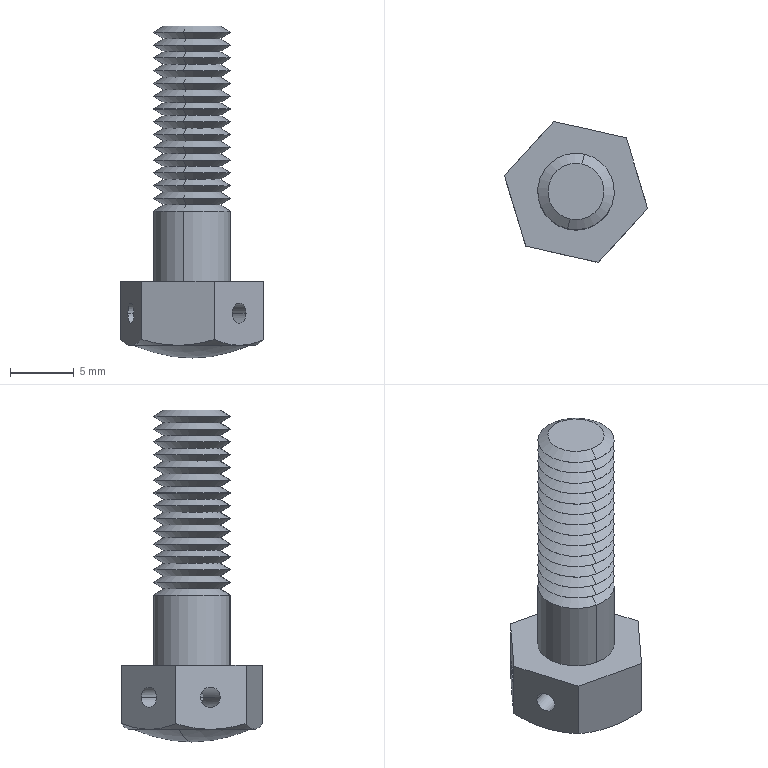Part | SolidWorks | features BaseBody 1 | 1 solid | 113 faces | box 11.215 x 11.04 x 26 mm | volume 895.249 mm3 | cone 64 | cylinder 38 | plane 9 | sphere 2 | commonest cylinder face diameters 6 x30 1.6 x8